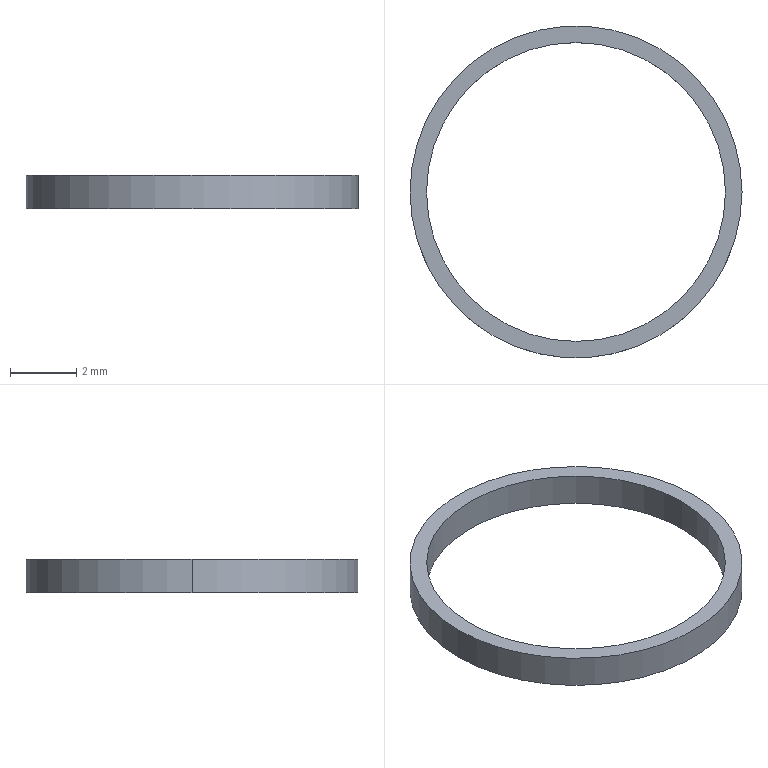Part | STEP file | Small spring | 1 solid | 6 faces | box 10 x 10 x 1 mm | volume 14.923 mm3 | cylinder 4 | plane 2 | commonest cylinder face diameters 9 x2 10 x2
STEP:
#1=CARTESIAN_POINT('',(0.,0.,0.));
#2=DIRECTION('',(0.,0.,1.));
#3=DIRECTION('',(1.,0.,0.));
#4=AXIS2_PLACEMENT_3D('',#1,#2,#3);
#5=CARTESIAN_POINT('',(-5.,0.,1.));
#6=VERTEX_POINT('',#5);
#7=CARTESIAN_POINT('',(5.,0.,1.));
#8=VERTEX_POINT('',#7);
#9=CARTESIAN_POINT('',(0.,0.,1.));
#10=DIRECTION('',(0.,0.,-1.));
#11=DIRECTION('',(-1.,0.,0.));
#12=AXIS2_PLACEMENT_3D('',#9,#10,#11);
#13=CIRCLE('',#12,5.);
#14=CARTESIAN_POINT('',(0.,0.,1.));
#15=DIRECTION('',(0.,0.,-1.));
#16=DIRECTION('',(-1.,0.,0.));
#17=AXIS2_PLACEMENT_3D('',#14,#15,#16);
#18=CYLINDRICAL_SURFACE('',#17,5.);
#19=CARTESIAN_POINT('',(0.,0.));
#20=DIRECTION('',(1.,0.));
#21=VECTOR('',#20,1.);
#22=LINE('',#19,#21);
#23=(GEOMETRIC_REPRESENTATION_CONTEXT(2)PARAMETRIC_REPRESENTATION_CONTEXT()REPRESENTATION_CONTEXT('',''));
#24=DEFINITIONAL_REPRESENTATION('',(#22),#23);
#25=PCURVE('',#18,#24);
#26=CARTESIAN_POINT('',(0.,0.,1.));
#27=DIRECTION('',(0.,0.,1.));
#28=DIRECTION('',(1.,0.,0.));
#29=AXIS2_PLACEMENT_3D('',#26,#27,#28);
#30=PLANE('',#29);
#31=CARTESIAN_POINT('',(-5.,0.));
#32=CARTESIAN_POINT('',(-5.,8.66));
#33=CARTESIAN_POINT('',(2.5,4.33));
#34=CARTESIAN_POINT('',(10.,0.));
#35=CARTESIAN_POINT('',(2.5,-4.33));
#36=CARTESIAN_POINT('',(-5.,-8.66));
#37=CARTESIAN_POINT('',(-5.,0.));
#38=(BOUNDED_CURVE()B_SPLINE_CURVE(2,(#31,#32,#33,#34,#35,#36,#37),.UNSPECIFIED.,.T.,.F.)B_SPLINE_CURVE_WITH_KNOTS((1,2,2,2,2,1),(-2.094,0.,2.094,4.189,6.283,8.378),.UNSPECIFIED.)CURVE()GEOMETRIC_REPRESENTATION_ITEM()RATIONAL_B_SPLINE_CURVE((1.,0.5,1.,0.5,1.,0.5,1.))REPRESENTATION_ITEM(''));
#39=(GEOMETRIC_REPRESENTATION_CONTEXT(2)PARAMETRIC_REPRESENTATION_CONTEXT()REPRESENTATION_CONTEXT('',''));
#40=DEFINITIONAL_REPRESENTATION('',(#38),#39);
#41=PCURVE('',#30,#40);
#42=SURFACE_CURVE('',#13,(#25,#41),.PCURVE_S1.);
#43=EDGE_CURVE('',#6,#8,#42,.T.);
#44=ORIENTED_EDGE('',*,*,#43,.T.);
#45=CARTESIAN_POINT('',(5.,0.,0.));
#46=VERTEX_POINT('',#45);
#47=CARTESIAN_POINT('',(5.,0.,1.));
#48=DIRECTION('',(0.,0.,-1.));
#49=VECTOR('',#48,1.);
#50=LINE('',#47,#49);
#51=CARTESIAN_POINT('',(3.142,0.));
#52=DIRECTION('',(0.,1.));
#53=VECTOR('',#52,1.);
#54=LINE('',#51,#53);
#55=(GEOMETRIC_REPRESENTATION_CONTEXT(2)PARAMETRIC_REPRESENTATION_CONTEXT()REPRESENTATION_CONTEXT('',''));
#56=DEFINITIONAL_REPRESENTATION('',(#54),#55);
#57=PCURVE('',#18,#56);
#58=CARTESIAN_POINT('',(0.,0.,1.));
#59=DIRECTION('',(0.,0.,-1.));
#60=DIRECTION('',(-1.,0.,0.));
#61=AXIS2_PLACEMENT_3D('',#58,#59,#60);
#62=CYLINDRICAL_SURFACE('',#61,5.);
#63=CARTESIAN_POINT('',(3.142,0.));
#64=DIRECTION('',(0.,1.));
#65=VECTOR('',#64,1.);
#66=LINE('',#63,#65);
#67=(GEOMETRIC_REPRESENTATION_CONTEXT(2)PARAMETRIC_REPRESENTATION_CONTEXT()REPRESENTATION_CONTEXT('',''));
#68=DEFINITIONAL_REPRESENTATION('',(#66),#67);
#69=PCURVE('',#62,#68);
#70=SURFACE_CURVE('',#50,(#57,#69),.PCURVE_S1.);
#71=EDGE_CURVE('',#8,#46,#70,.T.);
#72=ORIENTED_EDGE('',*,*,#71,.T.);
#73=CARTESIAN_POINT('',(-5.,0.,0.));
#74=VERTEX_POINT('',#73);
#75=CARTESIAN_POINT('',(0.,0.,0.));
#76=DIRECTION('',(0.,0.,1.));
#77=DIRECTION('',(-1.,0.,0.));
#78=AXIS2_PLACEMENT_3D('',#75,#76,#77);
#79=CIRCLE('',#78,5.);
#80=CARTESIAN_POINT('',(6.283,1.));
#81=DIRECTION('',(-1.,0.));
#82=VECTOR('',#81,1.);
#83=LINE('',#80,#82);
#84=(GEOMETRIC_REPRESENTATION_CONTEXT(2)PARAMETRIC_REPRESENTATION_CONTEXT()REPRESENTATION_CONTEXT('',''));
#85=DEFINITIONAL_REPRESENTATION('',(#83),#84);
#86=PCURVE('',#18,#85);
#87=CARTESIAN_POINT('',(0.,0.,0.));
#88=DIRECTION('',(0.,0.,1.));
#89=DIRECTION('',(1.,0.,0.));
#90=AXIS2_PLACEMENT_3D('',#87,#88,#89);
#91=PLANE('',#90);
#92=CARTESIAN_POINT('',(0.,0.));
#93=DIRECTION('',(-1.,0.));
#94=AXIS2_PLACEMENT_2D('',#92,#93);
#95=CIRCLE('',#94,5.);
#96=(GEOMETRIC_REPRESENTATION_CONTEXT(2)PARAMETRIC_REPRESENTATION_CONTEXT()REPRESENTATION_CONTEXT('',''));
#97=DEFINITIONAL_REPRESENTATION('',(#95),#96);
#98=PCURVE('',#91,#97);
#99=SURFACE_CURVE('',#79,(#86,#98),.PCURVE_S1.);
#100=EDGE_CURVE('',#46,#74,#99,.T.);
#101=ORIENTED_EDGE('',*,*,#100,.T.);
#102=CARTESIAN_POINT('',(-5.,0.,1.));
#103=DIRECTION('',(0.,0.,-1.));
#104=VECTOR('',#103,1.);
#105=LINE('',#102,#104);
#106=CARTESIAN_POINT('',(0.,0.));
#107=DIRECTION('',(0.,1.));
#108=VECTOR('',#107,1.);
#109=LINE('',#106,#108);
#110=(GEOMETRIC_REPRESENTATION_CONTEXT(2)PARAMETRIC_REPRESENTATION_CONTEXT()REPRESENTATION_CONTEXT('',''));
#111=DEFINITIONAL_REPRESENTATION('',(#109),#110);
#112=PCURVE('',#18,#111);
#113=CARTESIAN_POINT('',(6.283,0.));
#114=DIRECTION('',(0.,1.));
#115=VECTOR('',#114,1.);
#116=LINE('',#113,#115);
#117=(GEOMETRIC_REPRESENTATION_CONTEXT(2)PARAMETRIC_REPRESENTATION_CONTEXT()REPRESENTATION_CONTEXT('',''));
#118=DEFINITIONAL_REPRESENTATION('',(#116),#117);
#119=PCURVE('',#62,#118);
#120=SURFACE_CURVE('',#105,(#112,#119),.PCURVE_S1.);
#121=EDGE_CURVE('',#6,#74,#120,.T.);
#122=ORIENTED_EDGE('',*,*,#121,.F.);
#123=EDGE_LOOP('',(#44,#72,#101,#122));
#124=FACE_BOUND('',#123,.T.);
#125=ADVANCED_FACE('',(#124),#18,.T.);
#126=CARTESIAN_POINT('',(-4.5,0.,1.));
#127=VERTEX_POINT('',#126);
#128=CARTESIAN_POINT('',(-4.5,0.,0.));
#129=VERTEX_POINT('',#128);
#130=CARTESIAN_POINT('',(-4.5,0.,1.));
#131=DIRECTION('',(0.,0.,-1.));
#132=VECTOR('',#131,1.);
#133=LINE('',#130,#132);
#134=CARTESIAN_POINT('',(0.,0.,1.));
#135=DIRECTION('',(0.,0.,-1.));
#136=DIRECTION('',(-1.,0.,0.));
#137=AXIS2_PLACEMENT_3D('',#134,#135,#136);
#138=CYLINDRICAL_SURFACE('',#137,4.5);
#139=CARTESIAN_POINT('',(6.283,0.));
#140=DIRECTION('',(0.,1.));
#141=VECTOR('',#140,1.);
#142=LINE('',#139,#141);
#143=(GEOMETRIC_REPRESENTATION_CONTEXT(2)PARAMETRIC_REPRESENTATION_CONTEXT()REPRESENTATION_CONTEXT('',''));
#144=DEFINITIONAL_REPRESENTATION('',(#142),#143);
#145=PCURVE('',#138,#144);
#146=CARTESIAN_POINT('',(0.,0.,1.));
#147=DIRECTION('',(0.,0.,-1.));
#148=DIRECTION('',(-1.,0.,0.));
#149=AXIS2_PLACEMENT_3D('',#146,#147,#148);
#150=CYLINDRICAL_SURFACE('',#149,4.5);
#151=CARTESIAN_POINT('',(0.,0.));
#152=DIRECTION('',(0.,1.));
#153=VECTOR('',#152,1.);
#154=LINE('',#151,#153);
#155=(GEOMETRIC_REPRESENTATION_CONTEXT(2)PARAMETRIC_REPRESENTATION_CONTEXT()REPRESENTATION_CONTEXT('',''));
#156=DEFINITIONAL_REPRESENTATION('',(#154),#155);
#157=PCURVE('',#150,#156);
#158=SURFACE_CURVE('',#133,(#145,#157),.PCURVE_S1.);
#159=EDGE_CURVE('',#127,#129,#158,.T.);
#160=ORIENTED_EDGE('',*,*,#159,.T.);
#161=CARTESIAN_POINT('',(4.5,0.,0.));
#162=VERTEX_POINT('',#161);
#163=CARTESIAN_POINT('',(0.,0.,0.));
#164=DIRECTION('',(0.,0.,-1.));
#165=DIRECTION('',(-1.,0.,0.));
#166=AXIS2_PLACEMENT_3D('',#163,#164,#165);
#167=CIRCLE('',#166,4.5);
#168=CARTESIAN_POINT('',(0.,1.));
#169=DIRECTION('',(1.,0.));
#170=VECTOR('',#169,1.);
#171=LINE('',#168,#170);
#172=(GEOMETRIC_REPRESENTATION_CONTEXT(2)PARAMETRIC_REPRESENTATION_CONTEXT()REPRESENTATION_CONTEXT('',''));
#173=DEFINITIONAL_REPRESENTATION('',(#171),#172);
#174=PCURVE('',#138,#173);
#175=CARTESIAN_POINT('',(-4.5,0.));
#176=CARTESIAN_POINT('',(-4.5,7.794));
#177=CARTESIAN_POINT('',(2.25,3.897));
#178=CARTESIAN_POINT('',(9.,0.));
#179=CARTESIAN_POINT('',(2.25,-3.897));
#180=CARTESIAN_POINT('',(-4.5,-7.794));
#181=CARTESIAN_POINT('',(-4.5,0.));
#182=(BOUNDED_CURVE()B_SPLINE_CURVE(2,(#175,#176,#177,#178,#179,#180,#181),.UNSPECIFIED.,.T.,.F.)B_SPLINE_CURVE_WITH_KNOTS((1,2,2,2,2,1),(-2.094,0.,2.094,4.189,6.283,8.378),.UNSPECIFIED.)CURVE()GEOMETRIC_REPRESENTATION_ITEM()RATIONAL_B_SPLINE_CURVE((1.,0.5,1.,0.5,1.,0.5,1.))REPRESENTATION_ITEM(''));
#183=(GEOMETRIC_REPRESENTATION_CONTEXT(2)PARAMETRIC_REPRESENTATION_CONTEXT()REPRESENTATION_CONTEXT('',''));
#184=DEFINITIONAL_REPRESENTATION('',(#182),#183);
#185=PCURVE('',#91,#184);
#186=SURFACE_CURVE('',#167,(#174,#185),.PCURVE_S1.);
#187=EDGE_CURVE('',#162,#129,#186,.T.);
#188=ORIENTED_EDGE('',*,*,#187,.F.);
#189=CARTESIAN_POINT('',(4.5,0.,1.));
#190=VERTEX_POINT('',#189);
#191=CARTESIAN_POINT('',(4.5,0.,1.));
#192=DIRECTION('',(0.,0.,-1.));
#193=VECTOR('',#192,1.);
#194=LINE('',#191,#193);
#195=CARTESIAN_POINT('',(3.142,0.));
#196=DIRECTION('',(0.,1.));
#197=VECTOR('',#196,1.);
#198=LINE('',#195,#197);
#199=(GEOMETRIC_REPRESENTATION_CONTEXT(2)PARAMETRIC_REPRESENTATION_CONTEXT()REPRESENTATION_CONTEXT('',''));
#200=DEFINITIONAL_REPRESENTATION('',(#198),#199);
#201=PCURVE('',#138,#200);
#202=CARTESIAN_POINT('',(3.142,0.));
#203=DIRECTION('',(0.,1.));
#204=VECTOR('',#203,1.);
#205=LINE('',#202,#204);
#206=(GEOMETRIC_REPRESENTATION_CONTEXT(2)PARAMETRIC_REPRESENTATION_CONTEXT()REPRESENTATION_CONTEXT('',''));
#207=DEFINITIONAL_REPRESENTATION('',(#205),#206);
#208=PCURVE('',#150,#207);
#209=SURFACE_CURVE('',#194,(#201,#208),.PCURVE_S1.);
#210=EDGE_CURVE('',#190,#162,#209,.T.);
#211=ORIENTED_EDGE('',*,*,#210,.F.);
#212=CARTESIAN_POINT('',(0.,0.,1.));
#213=DIRECTION('',(0.,0.,-1.));
#214=DIRECTION('',(-1.,0.,0.));
#215=AXIS2_PLACEMENT_3D('',#212,#213,#214);
#216=CIRCLE('',#215,4.5);
#217=CARTESIAN_POINT('',(0.,0.));
#218=DIRECTION('',(1.,0.));
#219=VECTOR('',#218,1.);
#220=LINE('',#217,#219);
#221=(GEOMETRIC_REPRESENTATION_CONTEXT(2)PARAMETRIC_REPRESENTATION_CONTEXT()REPRESENTATION_CONTEXT('',''));
#222=DEFINITIONAL_REPRESENTATION('',(#220),#221);
#223=PCURVE('',#138,#222);
#224=CARTESIAN_POINT('',(-4.5,0.));
#225=CARTESIAN_POINT('',(-4.5,7.794));
#226=CARTESIAN_POINT('',(2.25,3.897));
#227=CARTESIAN_POINT('',(9.,0.));
#228=CARTESIAN_POINT('',(2.25,-3.897));
#229=CARTESIAN_POINT('',(-4.5,-7.794));
#230=CARTESIAN_POINT('',(-4.5,0.));
#231=(BOUNDED_CURVE()B_SPLINE_CURVE(2,(#224,#225,#226,#227,#228,#229,#230),.UNSPECIFIED.,.T.,.F.)B_SPLINE_CURVE_WITH_KNOTS((1,2,2,2,2,1),(-2.094,0.,2.094,4.189,6.283,8.378),.UNSPECIFIED.)CURVE()GEOMETRIC_REPRESENTATION_ITEM()RATIONAL_B_SPLINE_CURVE((1.,0.5,1.,0.5,1.,0.5,1.))REPRESENTATION_ITEM(''));
#232=(GEOMETRIC_REPRESENTATION_CONTEXT(2)PARAMETRIC_REPRESENTATION_CONTEXT()REPRESENTATION_CONTEXT('',''));
#233=DEFINITIONAL_REPRESENTATION('',(#231),#232);
#234=PCURVE('',#30,#233);
#235=SURFACE_CURVE('',#216,(#223,#234),.PCURVE_S1.);
#236=EDGE_CURVE('',#190,#127,#235,.T.);
#237=ORIENTED_EDGE('',*,*,#236,.T.);
#238=EDGE_LOOP('',(#160,#188,#211,#237));
#239=FACE_BOUND('',#238,.F.);
#240=ADVANCED_FACE('',(#239),#138,.F.);
#241=ORIENTED_EDGE('',*,*,#71,.F.);
#242=CARTESIAN_POINT('',(0.,0.,1.));
#243=DIRECTION('',(0.,0.,-1.));
#244=DIRECTION('',(-1.,0.,0.));
#245=AXIS2_PLACEMENT_3D('',#242,#243,#244);
#246=CIRCLE('',#245,5.);
#247=CARTESIAN_POINT('',(0.,0.));
#248=DIRECTION('',(1.,0.));
#249=VECTOR('',#248,1.);
#250=LINE('',#247,#249);
#251=(GEOMETRIC_REPRESENTATION_CONTEXT(2)PARAMETRIC_REPRESENTATION_CONTEXT()REPRESENTATION_CONTEXT('',''));
#252=DEFINITIONAL_REPRESENTATION('',(#250),#251);
#253=PCURVE('',#62,#252);
#254=CARTESIAN_POINT('',(-5.,0.));
#255=CARTESIAN_POINT('',(-5.,8.66));
#256=CARTESIAN_POINT('',(2.5,4.33));
#257=CARTESIAN_POINT('',(10.,0.));
#258=CARTESIAN_POINT('',(2.5,-4.33));
#259=CARTESIAN_POINT('',(-5.,-8.66));
#260=CARTESIAN_POINT('',(-5.,0.));
#261=(BOUNDED_CURVE()B_SPLINE_CURVE(2,(#254,#255,#256,#257,#258,#259,#260),.UNSPECIFIED.,.T.,.F.)B_SPLINE_CURVE_WITH_KNOTS((1,2,2,2,2,1),(-2.094,0.,2.094,4.189,6.283,8.378),.UNSPECIFIED.)CURVE()GEOMETRIC_REPRESENTATION_ITEM()RATIONAL_B_SPLINE_CURVE((1.,0.5,1.,0.5,1.,0.5,1.))REPRESENTATION_ITEM(''));
#262=(GEOMETRIC_REPRESENTATION_CONTEXT(2)PARAMETRIC_REPRESENTATION_CONTEXT()REPRESENTATION_CONTEXT('',''));
#263=DEFINITIONAL_REPRESENTATION('',(#261),#262);
#264=PCURVE('',#30,#263);
#265=SURFACE_CURVE('',#246,(#253,#264),.PCURVE_S1.);
#266=EDGE_CURVE('',#8,#6,#265,.T.);
#267=ORIENTED_EDGE('',*,*,#266,.T.);
#268=ORIENTED_EDGE('',*,*,#121,.T.);
#269=CARTESIAN_POINT('',(0.,0.,0.));
#270=DIRECTION('',(0.,0.,1.));
#271=DIRECTION('',(-1.,0.,0.));
#272=AXIS2_PLACEMENT_3D('',#269,#270,#271);
#273=CIRCLE('',#272,5.);
#274=CARTESIAN_POINT('',(6.283,1.));
#275=DIRECTION('',(-1.,0.));
#276=VECTOR('',#275,1.);
#277=LINE('',#274,#276);
#278=(GEOMETRIC_REPRESENTATION_CONTEXT(2)PARAMETRIC_REPRESENTATION_CONTEXT()REPRESENTATION_CONTEXT('',''));
#279=DEFINITIONAL_REPRESENTATION('',(#277),#278);
#280=PCURVE('',#62,#279);
#281=CARTESIAN_POINT('',(0.,0.));
#282=DIRECTION('',(-1.,0.));
#283=AXIS2_PLACEMENT_2D('',#281,#282);
#284=CIRCLE('',#283,5.);
#285=(GEOMETRIC_REPRESENTATION_CONTEXT(2)PARAMETRIC_REPRESENTATION_CONTEXT()REPRESENTATION_CONTEXT('',''));
#286=DEFINITIONAL_REPRESENTATION('',(#284),#285);
#287=PCURVE('',#91,#286);
#288=SURFACE_CURVE('',#273,(#280,#287),.PCURVE_S1.);
#289=EDGE_CURVE('',#74,#46,#288,.T.);
#290=ORIENTED_EDGE('',*,*,#289,.T.);
#291=EDGE_LOOP('',(#241,#267,#268,#290));
#292=FACE_BOUND('',#291,.T.);
#293=ADVANCED_FACE('',(#292),#62,.T.);
#294=CARTESIAN_POINT('',(0.,0.,0.));
#295=DIRECTION('',(0.,0.,-1.));
#296=DIRECTION('',(-1.,0.,0.));
#297=AXIS2_PLACEMENT_3D('',#294,#295,#296);
#298=CIRCLE('',#297,4.5);
#299=CARTESIAN_POINT('',(-4.5,0.));
#300=CARTESIAN_POINT('',(-4.5,7.794));
#301=CARTESIAN_POINT('',(2.25,3.897));
#302=CARTESIAN_POINT('',(9.,0.));
#303=CARTESIAN_POINT('',(2.25,-3.897));
#304=CARTESIAN_POINT('',(-4.5,-7.794));
#305=CARTESIAN_POINT('',(-4.5,0.));
#306=(BOUNDED_CURVE()B_SPLINE_CURVE(2,(#299,#300,#301,#302,#303,#304,#305),.UNSPECIFIED.,.T.,.F.)B_SPLINE_CURVE_WITH_KNOTS((1,2,2,2,2,1),(-2.094,0.,2.094,4.189,6.283,8.378),.UNSPECIFIED.)CURVE()GEOMETRIC_REPRESENTATION_ITEM()RATIONAL_B_SPLINE_CURVE((1.,0.5,1.,0.5,1.,0.5,1.))REPRESENTATION_ITEM(''));
#307=(GEOMETRIC_REPRESENTATION_CONTEXT(2)PARAMETRIC_REPRESENTATION_CONTEXT()REPRESENTATION_CONTEXT('',''));
#308=DEFINITIONAL_REPRESENTATION('',(#306),#307);
#309=PCURVE('',#91,#308);
#310=CARTESIAN_POINT('',(0.,1.));
#311=DIRECTION('',(1.,0.));
#312=VECTOR('',#311,1.);
#313=LINE('',#310,#312);
#314=(GEOMETRIC_REPRESENTATION_CONTEXT(2)PARAMETRIC_REPRESENTATION_CONTEXT()REPRESENTATION_CONTEXT('',''));
#315=DEFINITIONAL_REPRESENTATION('',(#313),#314);
#316=PCURVE('',#150,#315);
#317=SURFACE_CURVE('',#298,(#309,#316),.PCURVE_S1.);
#318=EDGE_CURVE('',#129,#162,#317,.T.);
#319=ORIENTED_EDGE('',*,*,#318,.F.);
#320=ORIENTED_EDGE('',*,*,#187,.F.);
#321=EDGE_LOOP('',(#319,#320));
#322=FACE_BOUND('',#321,.T.);
#323=ORIENTED_EDGE('',*,*,#289,.F.);
#324=ORIENTED_EDGE('',*,*,#100,.F.);
#325=EDGE_LOOP('',(#323,#324));
#326=FACE_BOUND('',#325,.T.);
#327=ADVANCED_FACE('',(#322,#326),#91,.F.);
#328=CARTESIAN_POINT('',(0.,0.,1.));
#329=DIRECTION('',(0.,0.,-1.));
#330=DIRECTION('',(-1.,0.,0.));
#331=AXIS2_PLACEMENT_3D('',#328,#329,#330);
#332=CIRCLE('',#331,4.5);
#333=CARTESIAN_POINT('',(-4.5,0.));
#334=CARTESIAN_POINT('',(-4.5,7.794));
#335=CARTESIAN_POINT('',(2.25,3.897));
#336=CARTESIAN_POINT('',(9.,0.));
#337=CARTESIAN_POINT('',(2.25,-3.897));
#338=CARTESIAN_POINT('',(-4.5,-7.794));
#339=CARTESIAN_POINT('',(-4.5,0.));
#340=(BOUNDED_CURVE()B_SPLINE_CURVE(2,(#333,#334,#335,#336,#337,#338,#339),.UNSPECIFIED.,.T.,.F.)B_SPLINE_CURVE_WITH_KNOTS((1,2,2,2,2,1),(-2.094,0.,2.094,4.189,6.283,8.378),.UNSPECIFIED.)CURVE()GEOMETRIC_REPRESENTATION_ITEM()RATIONAL_B_SPLINE_CURVE((1.,0.5,1.,0.5,1.,0.5,1.))REPRESENTATION_ITEM(''));
#341=(GEOMETRIC_REPRESENTATION_CONTEXT(2)PARAMETRIC_REPRESENTATION_CONTEXT()REPRESENTATION_CONTEXT('',''));
#342=DEFINITIONAL_REPRESENTATION('',(#340),#341);
#343=PCURVE('',#30,#342);
#344=CARTESIAN_POINT('',(0.,0.));
#345=DIRECTION('',(1.,0.));
#346=VECTOR('',#345,1.);
#347=LINE('',#344,#346);
#348=(GEOMETRIC_REPRESENTATION_CONTEXT(2)PARAMETRIC_REPRESENTATION_CONTEXT()REPRESENTATION_CONTEXT('',''));
#349=DEFINITIONAL_REPRESENTATION('',(#347),#348);
#350=PCURVE('',#150,#349);
#351=SURFACE_CURVE('',#332,(#343,#350),.PCURVE_S1.);
#352=EDGE_CURVE('',#127,#190,#351,.T.);
#353=ORIENTED_EDGE('',*,*,#352,.T.);
#354=ORIENTED_EDGE('',*,*,#236,.T.);
#355=EDGE_LOOP('',(#353,#354));
#356=FACE_BOUND('',#355,.T.);
#357=ORIENTED_EDGE('',*,*,#43,.F.);
#358=ORIENTED_EDGE('',*,*,#266,.F.);
#359=EDGE_LOOP('',(#357,#358));
#360=FACE_BOUND('',#359,.T.);
#361=ADVANCED_FACE('',(#356,#360),#30,.T.);
#362=ORIENTED_EDGE('',*,*,#318,.F.);
#363=ORIENTED_EDGE('',*,*,#159,.F.);
#364=ORIENTED_EDGE('',*,*,#352,.T.);
#365=ORIENTED_EDGE('',*,*,#210,.T.);
#366=EDGE_LOOP('',(#362,#363,#364,#365));
#367=FACE_BOUND('',#366,.F.);
#368=ADVANCED_FACE('',(#367),#150,.F.);
#369=CLOSED_SHELL('',(#125,#240,#293,#327,#361,#368));
#370=MANIFOLD_SOLID_BREP('',#369);
#371=(LENGTH_UNIT()NAMED_UNIT(*)SI_UNIT(.MILLI.,.METRE.));
#372=UNCERTAINTY_MEASURE_WITH_UNIT(LENGTH_MEASURE(0.0000001),#371,'','');
#373=(NAMED_UNIT(*)PLANE_ANGLE_UNIT()SI_UNIT($,.RADIAN.));
#374=(NAMED_UNIT(*)SI_UNIT($,.STERADIAN.)SOLID_ANGLE_UNIT());
#375=(GEOMETRIC_REPRESENTATION_CONTEXT(3)GLOBAL_UNCERTAINTY_ASSIGNED_CONTEXT((#372))GLOBAL_UNIT_ASSIGNED_CONTEXT((#371,#373,#374))REPRESENTATION_CONTEXT('',''));
#376=ADVANCED_BREP_SHAPE_REPRESENTATION('',(#4,#370),#375);